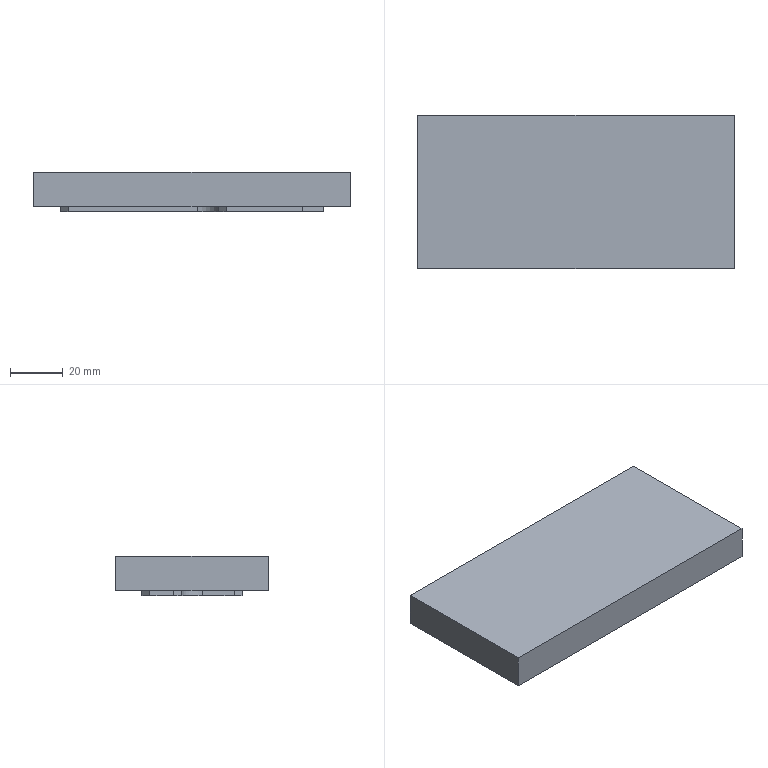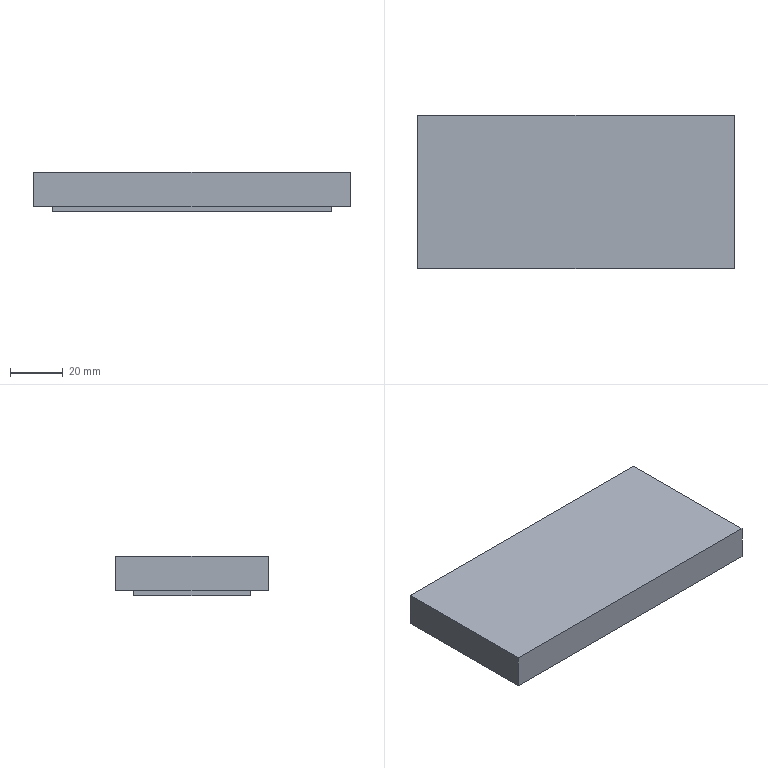CAM job | NX | 3-axis milling, drilling | part box 120 x 58 x 15 mm | stock box 120 x 58 x 15 mm
Tools:
number,name,description,diameter,corner_radius,flute_length,length,flutes
3,D63,Milling Tool-5 Parameters,63.0,0.0,50.0,75.0,2
1,D6A45,Milling Tool-5 Parameters,6.0,0.0,3.0,3.0,2
4,D10,Milling Tool-5 Parameters,10.0,0.0,50.0,75.0,2
16,D6JING,Milling Tool-5 Parameters,6.0,0.0,50.0,75.0,2
17,D3,Milling Tool-5 Parameters,3.0,0.0,50.0,75.0,2
13,3.4ZT,Drilling Tool,3.4,0.0,35.0,50.0,2
Operations:
program,operation,operation_type,tool,method,geometry_group,spindle_rpm,surface_speed,feed_per_tooth,feed_cut,feed_plunge,cut_length_mm,path_length_mm,cut_time_min,machine_time_min
1,FLOOR_WALL_COPY,VolumeBased25DMillingOperation,D63,METHOD,A,6500.0,1286.0,0.0962,1250.0,100.0,174.998,228.998,0.14,0.1454
1,DRILLING_COPY_1,Operation,D6A45,METHOD,A,5000.0,94.0,0.025,250.0,0.0,4.0,68.0,0.016,0.0224
1,DRILLING_COPY_1_COPY,Operation,3.4ZT,METHOD,A,2000.0,21.0,0.0375,150.0,0.0,10.521,81.043,0.0701,0.0772
1,ADAPTIVE_MILLING_COPY,CavityMilling,D10,METHOD,A,9500.0,298.0,0.1842,3500.0,1000.0,4244.438,4310.438,1.213,1.22
1,ZLEVEL_PROFILE_1_COPY,ZLevelMilling,D6JING,METHOD,A,9500.0,298.0,0.0526,1000.0,100.0,280.651,348.651,0.2807,0.2875
1,ZLEVEL_PROFILE_COPY_COPY_COPY,ZLevelMilling,D3,METHOD,A,9500.0,89.0,0.0632,1200.0,1000.0,4929.397,5105.006,4.115,4.133
1,11_COPY_COPY,ZLevelMilling,D6A45,METHOD,A,9500.0,179.0,0.0526,1000.0,100.0,503.333,830.907,0.5033,0.5361
2,ZLEVEL_PROFILE_1_COPY_COPY,ZLevelMilling,D10,METHOD,B,9500.0,298.0,0.1053,2000.0,100.0,577.496,639.496,0.2887,0.2949
2,FLOOR_WALL_COPY_COPY,VolumeBased25DMillingOperation,D63,METHOD,B,6500.0,1286.0,0.0962,1250.0,100.0,524.994,1018.99,0.42,0.4694
2,11_COPY_COPY_COPY,ZLevelMilling,D6A45,METHOD,B,9500.0,179.0,0.0526,1000.0,100.0,503.333,900.508,0.5033,0.5431
3,DRILLING_COPY_1_COPY_1,Operation,D6A45,METHOD,C,5000.0,94.0,0.01,100.0,0.0,50.0,329.855,0.5,0.528
3,ADAPTIVE_MILLING_COPY_COPY,CavityMilling,D10,METHOD,C,9500.0,298.0,0.1842,3500.0,1000.0,4232.947,4292.947,1.465,1.471
3,ADAPTIVE_MILLING_COPY_COPY_COPY,CavityMilling,D6JING,METHOD,C,9500.0,179.0,0.0789,1500.0,1000.0,234.912,687.283,0.1583,0.2035
3,FLOOR_WALL,VolumeBased25DMillingOperation,D6JING,METHOD,C,9500.0,179.0,0.0658,1250.0,100.0,930.794,996.794,0.7446,0.7512
3,11_COPY_COPY_COPY_COPY,ZLevelMilling,D6A45,METHOD,C,9500.0,179.0,0.0526,1000.0,100.0,273.763,329.763,0.2738,0.2794
3,刀补16,VolumeBased25DMillingOperation,D6JING,METHOD,C,9500.0,179.0,0.0658,1250.0,100.0,252.352,318.352,0.2019,0.2085